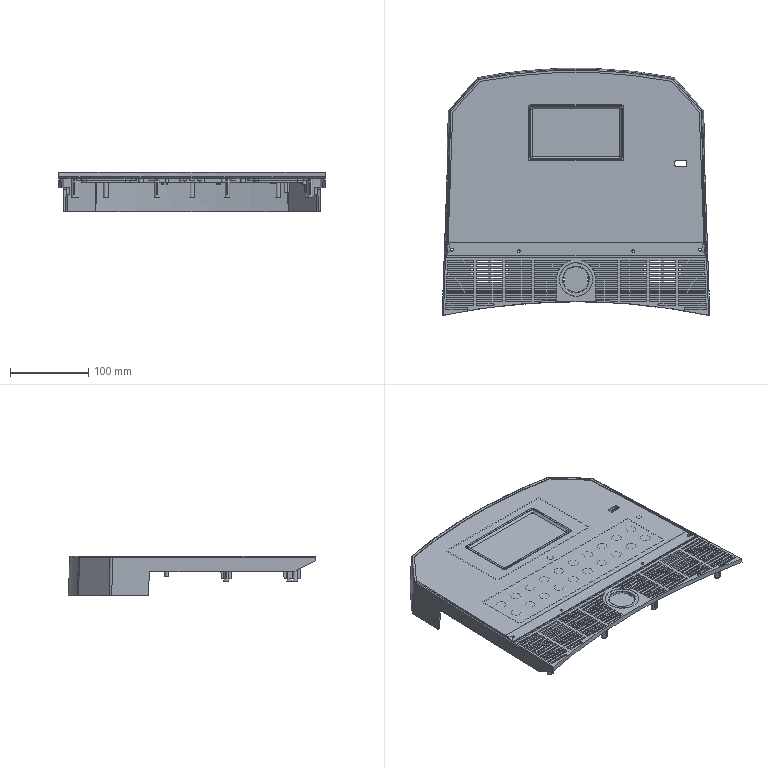Part | STEP file | 5091205W | 1 solid | 1501 faces | box 340.656 x 315.859 x 50.2 mm | volume 442857 mm3 | plane 1129 | cylinder 203 | cone 138 | spline 31 | commonest cylinder face diameters 2.3 x51 6 x47 1.7 x14 5 x14 7 x12 48.678 x12